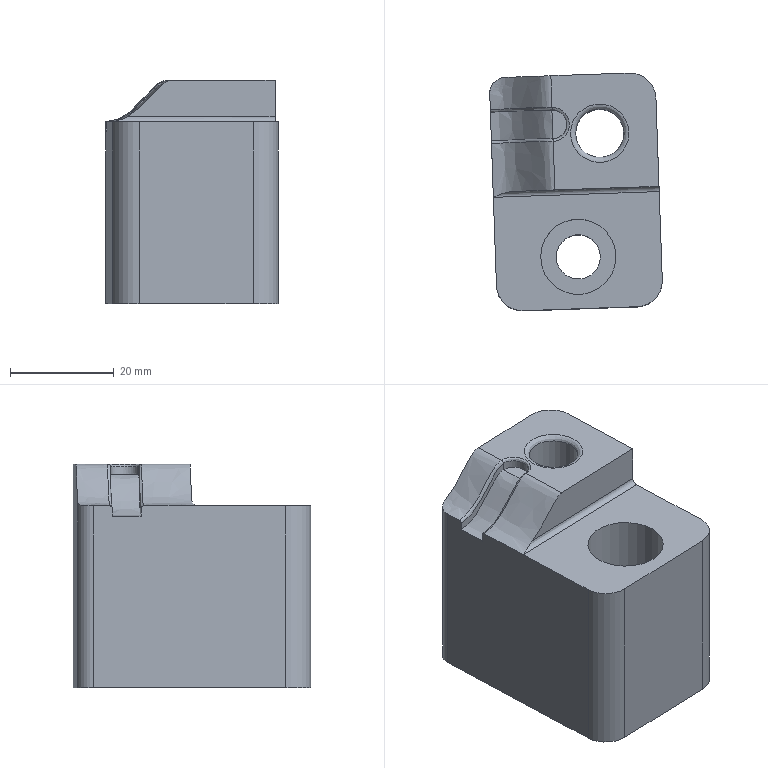Part | NX | features DIE-61 2 | 1 solid | 30 faces | box 33.223 x 45.745 x 43 mm | volume 46952 mm3 | plane 11 | cylinder 9 | spline 9 | torus 1 | commonest cylinder face diameters 10 x3 2 x1 6 x1 8.5 x1 9.27 x1 14 x1